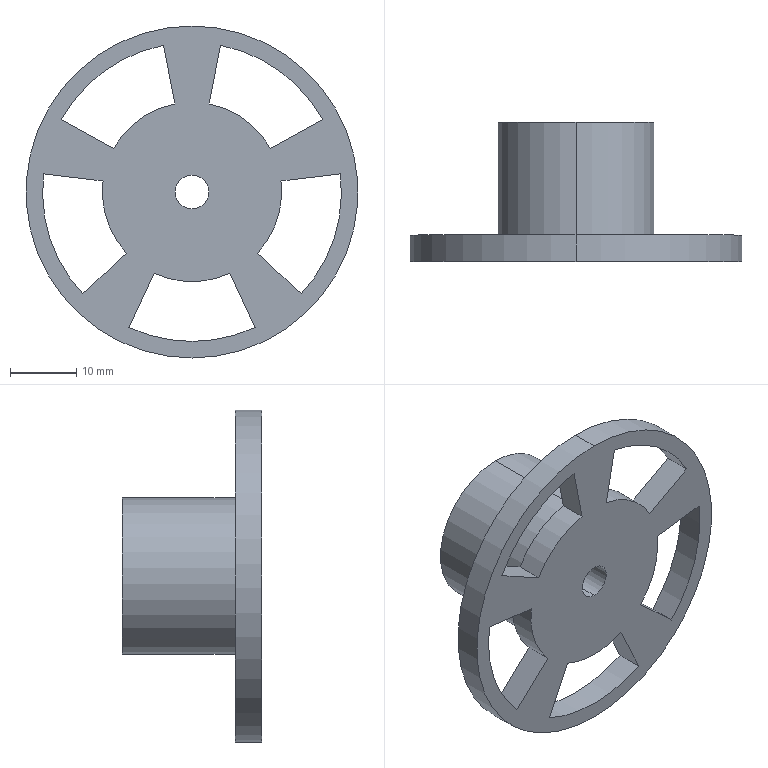Part | STEP file | Packing half-frame | 1 solid | 32 faces | box 50 x 21 x 50 mm | volume 8229 mm3 | cylinder 18 | plane 14 | commonest cylinder face diameters 27 x5 45 x5 5.1 x2 17.5 x2 23.5 x2 50 x2